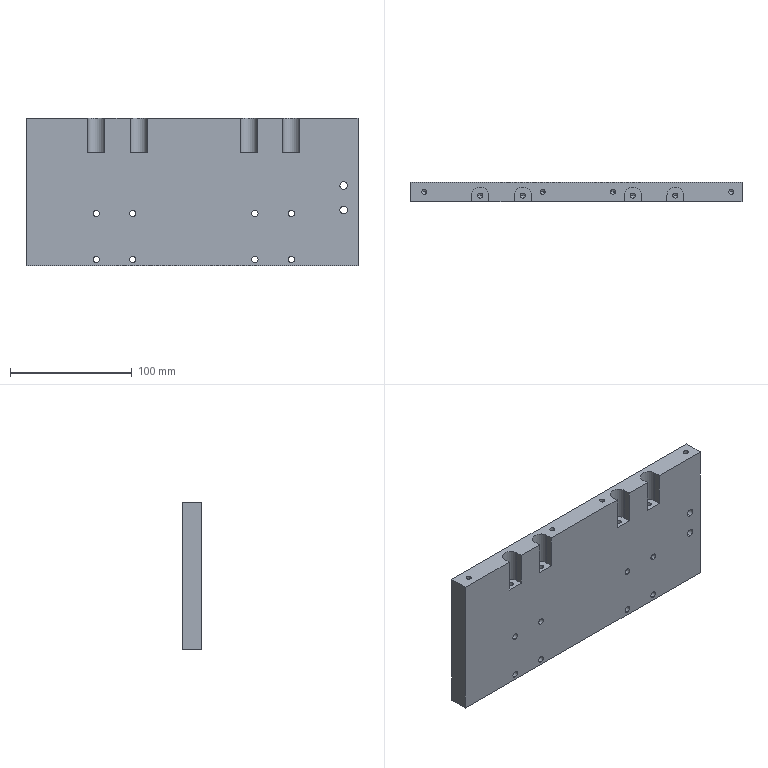Part | 1 solid | 98 faces | box 273 x 16 x 121.5 mm | volume 506434 mm3 | cylinder 56 | plane 26 | cone 16 | commonest cylinder face diameters 4.2 x16 5.2 x16 9 x16 6.2 x4 14 x4